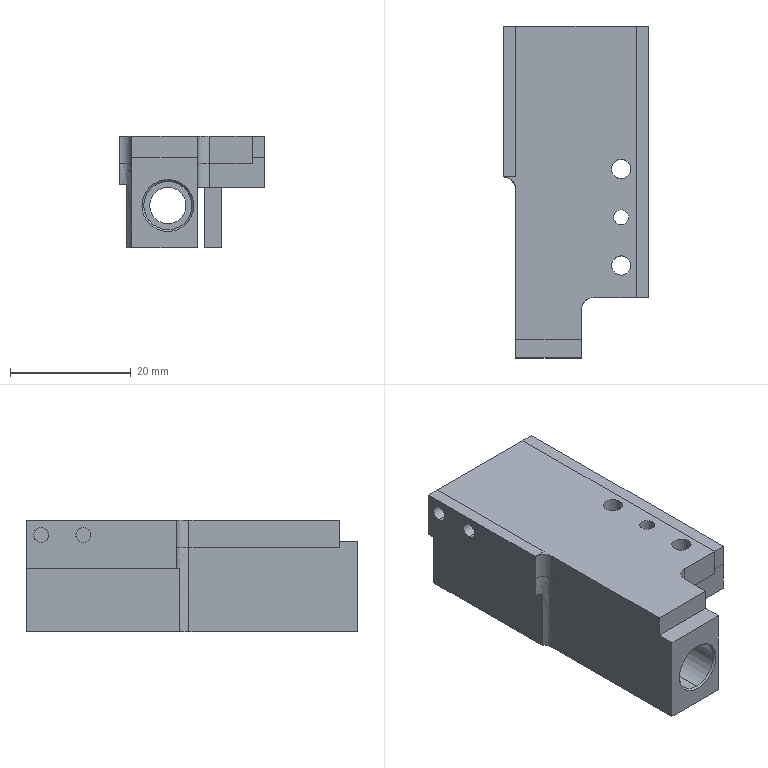NC program | NX | posted with a generic post | part box 24.15 x 55 x 18.5 mm
Lines 1 to 1747 of 2652:
N10 G17 G21 G94 G90
(FLOOR_WALL_COPY , TOOL : D63)
N12 T01 M6
N14 G54
N16 G17 G0 G90 X91.5 Y12.075 B0. C0. S6500 M3
N18 G43 Z30. H1
N20 Z8.571
N22 G94 G1 Z5.571 F1500.
N24 X86.5
N26 X-31.5
N28 X-36.5
N30 Z8.571
N32 G0 Z30.
N34 X91.5
N36 Z7.643
N38 G1 Z4.643
N40 X86.5
N42 X-31.5
N44 X-36.5
N46 Z7.643
N48 G0 Z30.
N50 X91.5
N52 Z6.714
N54 G1 Z3.714
N56 X86.5
N58 X-31.5
N60 X-36.5
N62 Z6.714
N64 G0 Z30.
N66 X91.5
N68 Z5.786
N70 G1 Z2.786
N72 X86.5
N74 X-31.5
N76 X-36.5
N78 Z5.786
N80 G0 Z30.
N82 X91.5
N84 Z4.857
N86 G1 Z1.857
N88 X86.5
N90 X-31.5
N92 X-36.5
N94 Z4.857
N96 G0 Z30.
N98 X91.5
N100 Z3.929
N102 G1 Z0.929
N104 X86.5
N106 X-31.5
N108 X-36.5
N110 Z3.929
N112 G0 Z30.
N114 X91.5
N116 Z3.
N118 G1 Z0.
N120 X86.5
N122 X-31.5
N124 X-36.5
N126 Z3.
N128 G0 Z30.
N130 M5
(FLOOR_WALL_1 , TOOL : D10)
N132 T10 M6
N134 G54
N136 G17 G0 G90 X34.979 Y-6. B0. C0. S9500 M3
N138 G43 Z30. H10
N140 Z-0.99
N142 G94 G1 X34.691 Y-5.5 F1000.
N144 G3 X33.825 Y-5. R1.
N146 G1 X-5. F3000.
N148 Y2.075
N150 X18.1
N152 Y6.075
N154 X50.
N156 Y-5.
N158 X33.825
N160 Y0.
N162 X22.649
N164 G3 X22.999 Y1.075 R5.
N166 G1 X45.
N168 Y0.
N170 X33.825
N172 G3 X32.959 Y-0.5 R1.
N174 G0 Z30.
N176 X34.979 Y-6.
N178 Z-1.98
N180 G1 X34.691 Y-5.5 F1000.
N182 G3 X33.825 Y-5. R1.
N184 G1 X-5. F3000.
N186 Y2.075
N188 X18.1
N190 Y6.075
N192 X50.
N194 Y-5.
N196 X33.825
N198 Y0.
N200 X22.649
N202 G3 X22.999 Y1.075 R5.
N204 G1 X45.
N206 Y0.
N208 X33.825
N210 G3 X32.959 Y-0.5 R1.
N212 G0 Z30.
N214 X34.979 Y-6.
N216 Z-2.97
N218 G1 X34.691 Y-5.5 F1000.
N220 G3 X33.825 Y-5. R1.
N222 G1 X-5. F3000.
N224 Y2.075
N226 X18.1
N228 Y6.075
N230 X50.
N232 Y-5.
N234 X33.825
N236 Y0.
N238 X22.649
N240 G3 X22.999 Y1.075 R5.
N242 G1 X45.
N244 Y0.
N246 X33.825
N248 G3 X32.959 Y-0.5 R1.
N250 G0 Z30.
N252 X34.979 Y-6.
N254 Z-3.96
N256 G1 X34.691 Y-5.5 F1000.
N258 G3 X33.825 Y-5. R1.
N260 G1 X-5. F3000.
N262 Y2.075
N264 X18.1
N266 Y6.075
N268 X50.
N270 Y-5.
N272 X33.825
N274 Y0.
N276 X22.649
N278 G3 X22.999 Y1.075 R5.
N280 G1 X45.
N282 Y0.
N284 X33.825
N286 G3 X32.959 Y-0.5 R1.
N288 G0 Z30.
N290 X34.979 Y-6.
N292 Z-4.95
N294 G1 X34.691 Y-5.5 F1000.
N296 G3 X33.825 Y-5. R1.
N298 G1 X-5. F3000.
N300 Y2.075
N302 X18.1
N304 Y6.075
N306 X50.
N308 Y-5.
N310 X33.825
N312 Y0.
N314 X22.649
N316 G3 X22.999 Y1.075 R5.
N318 G1 X45.
N320 Y0.
N322 X33.825
N324 G3 X32.959 Y-0.5 R1.
N326 G0 Z30.
N328 X34.979 Y-6.
N330 Z-5.94
N332 G1 X34.691 Y-5.5 F1000.
N334 G3 X33.825 Y-5. R1.
N336 G1 X-5. F3000.
N338 Y2.075
N340 X18.1
N342 Y6.075
N344 X50.
N346 Y-5.
N348 X33.825
N350 Y0.
N352 X22.649
N354 G3 X22.999 Y1.075 R5.
N356 G1 X45.
N358 Y0.
N360 X33.825
N362 G3 X32.959 Y-0.5 R1.
N364 G0 Z30.
N366 X34.979 Y-6.
N368 Z-6.93
N370 G1 X34.691 Y-5.5 F1000.
N372 G3 X33.825 Y-5. R1.
N374 G1 X-5. F3000.
N376 Y2.075
N378 X18.1
N380 Y6.075
N382 X50.
N384 Y-5.
N386 X33.825
N388 Y0.
N390 X22.649
N392 G3 X22.999 Y1.075 R5.
N394 G1 X45.
N396 Y0.
N398 X33.825
N400 G3 X32.959 Y-0.5 R1.
N402 G0 Z30.
N404 X34.979 Y-6.
N406 Z-7.92
N408 G1 X34.691 Y-5.5 F1000.
N410 G3 X33.825 Y-5. R1.
N412 G1 X-5. F3000.
N414 Y2.075
N416 X18.1
N418 Y6.075
N420 X50.
N422 Y-5.
N424 X33.825
N426 Y0.
N428 X22.649
N430 G3 X22.999 Y1.075 R5.
N432 G1 X45.
N434 Y0.
N436 X33.825
N438 G3 X32.959 Y-0.5 R1.
N440 G0 Z30.
N442 X34.979 Y-6.
N444 Z-8.91
N446 G1 X34.691 Y-5.5 F1000.
N448 G3 X33.825 Y-5. R1.
N450 G1 X-5. F3000.
N452 Y2.075
N454 X18.1
N456 Y6.075
N458 X50.
N460 Y-5.
N462 X33.825
N464 Y0.
N466 X22.649
N468 G3 X22.999 Y1.075 R5.
N470 G1 X45.
N472 Y0.
N474 X33.825
N476 G3 X32.959 Y-0.5 R1.
N478 G0 Z30.
N480 X34.979 Y-6.
N482 Z-9.9
N484 G1 X34.691 Y-5.5 F1000.
N486 G3 X33.825 Y-5. R1.
N488 G1 X-5. F3000.
N490 Y2.075
N492 X18.1
N494 Y6.075
N496 X50.
N498 Y-5.
N500 X33.825
N502 Y0.
N504 X22.649
N506 G3 X22.999 Y1.075 R5.
N508 G1 X45.
N510 Y0.
N512 X33.825
N514 G3 X32.959 Y-0.5 R1.
N516 G0 Z30.
(CAVITY_MILL , TOOL : D10)
N518 X-6.064 Y16.076
N520 Z0.5
N522 G1 Z-1. F1000.
N524 X-0.56 Y16.941
N526 G2 X-0.06 Y16.075 R1.
N528 G1 Y15.175 F3000.
N530 X13.
N532 X13.264 Y15.168
N534 G2 X13.773 Y15.116 R5.1
N536 G1 X15.811
N538 X15.812 Y14.989
N540 X15.84 Y14.816
N542 Y14.542
N544 Y14.38
N546 X15.826
N548 X15.784 Y14.399
N550 X15.777 Y14.352
N552 X15.9 Y14.27
N554 Y16.975
N556 X-0.06
N558 Y16.075
N560 G2 X-0.56 Y15.209 R1.
N562 G1 X-6.064 Y16.076
N564 Z0.5
N566 G0 X-6.065 Z-0.5
N568 G1 Z-2. F1000.
N570 X-0.56 Y16.941
N572 G2 X-0.06 Y16.075 R1.
N574 G1 Y15.175 F3000.
N576 X13.
N578 X13.264 Y15.168
N580 G2 X13.773 Y15.116 R5.1
N582 G1 X15.811
N584 X15.812 Y14.989
N586 X15.84 Y14.816
N588 Y14.542
N590 Y14.38
N592 X15.826
N594 X15.784 Y14.399
N596 X15.777 Y14.353
N598 X15.9 Y14.27
N600 Y16.975
N602 X-0.06
N604 Y16.075
N606 G2 X-0.56 Y15.209 R1.
N608 G1 X-6.065 Y16.076
N610 Z-0.5
N612 G0 X-6.067 Z-1.5
N614 G1 Z-3. F1000.
N616 X-0.56 Y16.941
N618 G2 X-0.06 Y16.075 R1.
N620 G1 Y15.175 F3000.
N622 X13.
N624 X13.264 Y15.168
N626 G2 X13.773 Y15.116 R5.1
N628 G1 X15.811
N630 X15.812 Y14.989
N632 X15.84 Y14.816
N634 Y14.542
N636 Y14.38
N638 X15.826
N640 X15.784 Y14.399
N642 X15.777 Y14.353
N644 X15.9 Y14.27
N646 Y16.975
N648 X-0.06
N650 Y16.075
N652 G2 X-0.56 Y15.209 R1.
N654 G1 X-6.067 Y16.076
N656 Z-1.5
N658 G0 X-6.069 Z-2.5
N660 G1 Z-4. F1000.
N662 X-0.56 Y16.941
N664 G2 X-0.06 Y16.075 R1.
N666 G1 Y15.175 F3000.
N668 X13.
N670 X13.264 Y15.168
N672 G2 X13.773 Y15.116 R5.1
N674 G1 X15.811
N676 X15.812 Y14.989
N678 X15.84 Y14.816
N680 Y14.542
N682 Y14.38
N684 X15.826
N686 X15.784 Y14.399
N688 X15.777 Y14.353
N690 X15.9 Y14.271
N692 Y16.975
N694 X-0.06
N696 Y16.075
N698 G2 X-0.56 Y15.209 R1.
N700 G1 X-6.069 Y16.076
N702 Z-2.5
N704 G0 X-6.07 Z-3.5
N706 G1 Z-5. F1000.
N708 X-0.56 Y16.941
N710 G2 X-0.06 Y16.075 R1.
N712 G1 Y15.175 F3000.
N714 X13.
N716 X13.216 Y15.173
N718 X13.264 Y15.168
N720 G2 X13.773 Y15.116 R5.1
N722 G1 X15.811
N724 X15.812 Y14.989
N726 X15.84 Y14.816
N728 Y14.542
N730 Y14.38
N732 X15.826
N734 X15.784 Y14.399
N736 X15.777 Y14.353
N738 X15.899 Y14.271
N740 X15.9 Y16.975
N742 X-0.06
N744 Y16.075
N746 G2 X-0.56 Y15.209 R1.
N748 G1 X-6.07 Y16.076
N750 Z-3.5
N752 G0 X-6.072 Z-4.5
N754 G1 Z-6. F1000.
N756 X-0.56 Y16.941
N758 G2 X-0.06 Y16.075 R1.
N760 G1 Y15.175 F3000.
N762 X13.
N764 X13.216 Y15.173
N766 X13.264 Y15.168
N768 G2 X13.773 Y15.116 R5.1
N770 G1 X15.811
N772 X15.812 Y14.989
N774 X15.84 Y14.816
N776 Y14.542
N778 Y14.38
N780 X15.826
N782 X15.784 Y14.399
N784 X15.777 Y14.353
N786 X15.899 Y14.272
N788 Y16.975
N790 X-0.06
N792 Y16.075
N794 G2 X-0.56 Y15.209 R1.
N796 G1 X-6.072 Y16.076
N798 Z-4.5
N800 G0 X-6.073 Z-5.5
N802 G1 Z-7. F1000.
N804 X-0.56 Y16.941
N806 G2 X-0.06 Y16.075 R1.
N808 G1 Y15.175 F3000.
N810 X13.
N812 X13.216 Y15.174
N814 X13.264 Y15.168
N816 G2 X13.773 Y15.116 R5.1
N818 G1 X15.811
N820 X15.812 Y14.989
N822 X15.84 Y14.816
N824 Y14.542
N826 Y14.38
N828 X15.826
N830 X15.784 Y14.399
N832 X15.777 Y14.353
N834 X15.899 Y14.273
N836 Y16.975
N838 X-0.06
N840 Y16.075
N842 G2 X-0.56 Y15.209 R1.
N844 G1 X-6.073 Y16.076
N846 Z-5.5
N848 G0 X-6.075 Z-6.5
N850 G1 Z-8. F1000.
N852 X-0.56 Y16.941
N854 G2 X-0.06 Y16.075 R1.
N856 G1 Y15.175 F3000.
N858 X13.
N860 X13.216 Y15.174
N862 X13.264 Y15.168
N864 G2 X13.773 Y15.116 R5.1
N866 G1 X15.811
N868 X15.812 Y14.989
N870 X15.84 Y14.816
N872 Y14.542
N874 Y14.38
N876 X15.826
N878 X15.784 Y14.399
N880 X15.777 Y14.353
N882 X15.898 Y14.273
N884 X15.899 Y16.975
N886 X-0.06
N888 Y16.075
N890 G2 X-0.56 Y15.209 R1.
N892 G1 X-6.075 Y16.076
N894 Z-6.5
N896 G0 X-6.076 Z-7.5
N898 G1 Z-9. F1000.
N900 X-0.56 Y16.941
N902 G2 X-0.06 Y16.075 R1.
N904 G1 Y15.175 F3000.
N906 X13.
N908 X13.216
N910 X13.264 Y15.168
N912 G2 X13.773 Y15.116 R5.1
N914 G1 X15.811
N916 X15.812 Y14.989
N918 X15.84 Y14.816
N920 Y14.542
N922 Y14.38
N924 X15.826
N926 X15.784 Y14.399
N928 X15.777 Y14.353
N930 X15.898 Y14.274
N932 X15.899 Y16.975
N934 X-0.06
N936 Y16.075
N938 G2 X-0.56 Y15.209 R1.
N940 G1 X-6.076 Y16.076
N942 Z-7.5
N944 G0 X-6.078 Z-8.5
N946 G1 Z-10. F1000.
N948 X-0.56 Y16.941
N950 G2 X-0.06 Y16.075 R1.
N952 G1 Y15.175 F3000.
N954 X13.288
N956 X15.9
N958 X15.899 Y16.975
N960 X-0.06
N962 Y16.075
N964 G2 X-0.56 Y15.209 R1.
N966 G1 X-6.078 Y16.076
N968 Z-8.5
N970 G0 X-6.079 Z-9.45
N972 G1 Z-10.95 F1000.
N974 X-0.56 Y16.941
N976 G2 X-0.06 Y16.075 R1.
N978 G1 Y15.175 F3000.
N980 X15.9
N982 X15.899 Y16.975
N984 X-0.06
N986 Y16.075
N988 G2 X-0.56 Y15.209 R1.
N990 G1 X-6.079 Y16.076
N992 Z-9.45
N994 G0 X-6.081 Z-10.4
N996 G1 Z-11.9 F1000.
N998 X-0.56 Y16.941
N1000 G2 X-0.06 Y16.075 R1.
N1002 G1 Y15.175 F3000.
N1004 X15.9
N1006 X15.899 Y16.975
N1008 X-0.06
N1010 Y16.075
N1012 G2 X-0.56 Y15.209 R1.
N1014 G1 X-6.081 Y16.076
N1016 Z-10.4
N1018 G0 Z30.
N1020 M5
(CAVITY_MILL_COPY , TOOL : D6)
N1022 T06 M6
N1024 G54
N1026 G17 G0 G90 X16.8 Y15.798 B0. C0. S9500 M3
N1028 G43 Z30. H6
N1030 Z0.5
N1032 G94 G1 Z-0.5 F1000.
N1034 X17.5 Y16.202
N1036 G3 X18. Y17.069 R1.
N1038 G1 Y19.075 F2000.
N1040 X15.994
N1042 G3 X15.127 Y18.575 R1.
N1044 G1 X14.723 Y17.875
N1046 Z0.5
N1048 G0 Z30.
N1050 X16.8 Y15.798
N1052 Z0.
N1054 G1 Z-1. F1000.
N1056 X17.5 Y16.202
N1058 G3 X18. Y17.068 R1.
N1060 G1 Y19.075 F2000.
N1062 X15.993
N1064 G3 X15.127 Y18.575 R1.
N1066 G1 X14.723 Y17.875
N1068 Z0.
N1070 G0 X16.8 Y15.798 Z-0.5
N1072 G1 Z-1.5 F1000.
N1074 X17.5 Y16.202
N1076 G3 X18. Y17.068 R1.
N1078 G1 Y19.075 F2000.
N1080 X15.993
N1082 G3 X15.127 Y18.575 R1.
N1084 G1 X14.723 Y17.875
N1086 Z-0.5
N1088 G0 X16.8 Y15.798 Z-1.
N1090 G1 Z-2. F1000.
N1092 X17.5 Y16.202
N1094 G3 X18. Y17.068 R1.
N1096 G1 Y19.075 F2000.
N1098 X15.993
N1100 G3 X15.127 Y18.575 R1.
N1102 G1 X14.723 Y17.875
N1104 Z-1.
N1106 G0 X16.8 Y15.798 Z-1.5
N1108 G1 Z-2.5 F1000.
N1110 X17.5 Y16.202
N1112 G3 X18. Y17.068 R1.
N1114 G1 Y19.075 F2000.
N1116 X15.993
N1118 G3 X15.127 Y18.575 R1.
N1120 G1 X14.723 Y17.875
N1122 Z-1.5
N1124 G0 X16.8 Y15.798 Z-2.
N1126 G1 Z-3. F1000.
N1128 X17.5 Y16.202
N1130 G3 X18. Y17.068 R1.
N1132 G1 Y19.075 F2000.
N1134 X15.993
N1136 G3 X15.127 Y18.575 R1.
N1138 G1 X14.723 Y17.875
N1140 Z-2.
N1142 G0 X16.8 Y15.798 Z-2.5
N1144 G1 Z-3.5 F1000.
N1146 X17.5 Y16.202
N1148 G3 X18. Y17.068 R1.
N1150 G1 Y19.075 F2000.
N1152 X15.993
N1154 G3 X15.127 Y18.575 R1.
N1156 G1 X14.723 Y17.875
N1158 Z-2.5
N1160 G0 X16.8 Y15.798 Z-3.
N1162 G1 Z-4. F1000.
N1164 X17.5 Y16.202
N1166 G3 X18. Y17.068 R1.
N1168 G1 Y19.075 F2000.
N1170 X15.993
N1172 G3 X15.127 Y18.575 R1.
N1174 G1 X14.723 Y17.875
N1176 Z-3.
N1178 G0 X16.8 Y15.798 Z-3.5
N1180 G1 Z-4.5 F1000.
N1182 X17.5 Y16.202
N1184 G3 X18. Y17.068 R1.
N1186 G1 Y19.075 F2000.
N1188 X15.993
N1190 G3 X15.127 Y18.575 R1.
N1192 G1 X14.723 Y17.875
N1194 Z-3.5
N1196 G0 X16.8 Y15.798 Z-4.
N1198 G1 Z-5. F1000.
N1200 X17.5 Y16.202
N1202 G3 X18. Y17.068 R1.
N1204 G1 Y19.075 F2000.
N1206 X15.993
N1208 G3 X15.127 Y18.575 R1.
N1210 G1 X14.723 Y17.875
N1212 Z-4.
N1214 G0 X16.8 Y15.798 Z-4.5
N1216 G1 Z-5.5 F1000.
N1218 X17.5 Y16.202
N1220 G3 X18. Y17.068 R1.
N1222 G1 Y19.075 F2000.
N1224 X15.993
N1226 G3 X15.127 Y18.575 R1.
N1228 G1 X14.723 Y17.875
N1230 Z-4.5
N1232 G0 X16.8 Y15.798 Z-5.
N1234 G1 Z-6. F1000.
N1236 X17.5 Y16.202
N1238 G3 X18. Y17.068 R1.
N1240 G1 Y19.075 F2000.
N1242 X15.993
N1244 G3 X15.127 Y18.575 R1.
N1246 G1 X14.723 Y17.875
N1248 Z-5.
N1250 G0 X16.8 Y15.798 Z-5.5
N1252 G1 Z-6.5 F1000.
N1254 X17.5 Y16.202
N1256 G3 X18. Y17.068 R1.
N1258 G1 Y19.075 F2000.
N1260 X15.993
N1262 G3 X15.127 Y18.575 R1.
N1264 G1 X14.723 Y17.875
N1266 Z-5.5
N1268 G0 X16.8 Y15.798 Z-6.
N1270 G1 Z-7. F1000.
N1272 X17.5 Y16.202
N1274 G3 X18. Y17.068 R1.
N1276 G1 Y19.075 F2000.
N1278 X15.993
N1280 G3 X15.127 Y18.575 R1.
N1282 G1 X14.723 Y17.875
N1284 Z-6.
N1286 G0 X16.8 Y15.798 Z-6.5
N1288 G1 Z-7.5 F1000.
N1290 X17.5 Y16.202
N1292 G3 X18. Y17.068 R1.
N1294 G1 Y19.075 F2000.
N1296 X15.993
N1298 G3 X15.127 Y18.575 R1.
N1300 G1 X14.723 Y17.875
N1302 Z-6.5
N1304 G0 X16.8 Y15.798 Z-7.
N1306 G1 Z-8. F1000.
N1308 X17.5 Y16.202
N1310 G3 X18. Y17.068 R1.
N1312 G1 Y19.075 F2000.
N1314 X15.993
N1316 G3 X15.127 Y18.575 R1.
N1318 G1 X14.723 Y17.875
N1320 Z-7.
N1322 G0 X16.8 Y15.798 Z-7.5
N1324 G1 Z-8.5 F1000.
N1326 X17.5 Y16.202
N1328 G3 X18. Y17.068 R1.
N1330 G1 Y19.075 F2000.
N1332 X15.993
N1334 G3 X15.127 Y18.575 R1.
N1336 G1 X14.723 Y17.875
N1338 Z-7.5
N1340 G0 X16.8 Y15.798 Z-8.
N1342 G1 Z-9. F1000.
N1344 X17.5 Y16.202
N1346 G3 X18. Y17.068 R1.
N1348 G1 Y19.075 F2000.
N1350 X15.993
N1352 G3 X15.127 Y18.575 R1.
N1354 G1 X14.723 Y17.875
N1356 Z-8.
N1358 G0 X16.8 Y15.798 Z-8.5
N1360 G1 Z-9.5 F1000.
N1362 X17.5 Y16.202
N1364 G3 X18. Y17.068 R1.
N1366 G1 Y19.075 F2000.
N1368 X15.993
N1370 G3 X15.127 Y18.575 R1.
N1372 G1 X14.723 Y17.875
N1374 Z-8.5
N1376 G0 X16.8 Y15.798 Z-9.
N1378 G1 Z-10. F1000.
N1380 X17.5 Y16.202
N1382 G3 X18. Y17.068 R1.
N1384 G1 Y19.075 F2000.
N1386 X15.993
N1388 G3 X15.127 Y18.575 R1.
N1390 G1 X14.723 Y17.875
N1392 Z-9.
N1394 G0 X16.8 Y15.797 Z-9.5
N1396 G1 Z-10.5 F1000.
N1398 X17.5 Y16.202
N1400 G3 X18. Y17.068 R1.
N1402 G1 Y19.075 F2000.
N1404 X15.993
N1406 G3 X15.127 Y18.575 R1.
N1408 G1 X14.722 Y17.875
N1410 Z-9.5
N1412 G0 X16.8 Y15.797 Z-10.
N1414 G1 Z-11. F1000.
N1416 X17.5 Y16.202
N1418 G3 X18. Y17.068 R1.
N1420 G1 Y19.075 F2000.
N1422 X15.993
N1424 G3 X15.127 Y18.575 R1.
N1426 G1 X14.722 Y17.875
N1428 Z-10.
N1430 G0 X16.8 Y15.797 Z-10.5
N1432 G1 Z-11.5 F1000.
N1434 X17.5 Y16.202
N1436 G3 X18. Y17.068 R1.
N1438 G1 Y19.075 F2000.
N1440 X15.993
N1442 G3 X15.127 Y18.575 R1.
N1444 G1 X14.722 Y17.875
N1446 Z-10.5
N1448 G0 X16.8 Y15.797 Z-11.
N1450 G1 Z-12. F1000.
N1452 X17.5 Y16.201
N1454 G3 X18. Y17.067 R1.
N1456 G1 Y19.075 F2000.
N1458 X15.992
N1460 G3 X15.126 Y18.575 R1.
N1462 G1 X14.722 Y17.875
N1464 Z-11.
N1466 G0 Z30.
N1468 X16.8 Y15.979
N1470 Z0.5
N1472 G1 Z-0.5 F1000.
N1474 X17.409 Y12.975
N1476 G2 X17.923 Y12.118 R1.
N1478 G1 X17.939 Y11.219 F2000.
N1480 X17.936 Y11.155
N1482 X18. Y11.16
N1484 Y14.082
N1486 G3 X17.515 Y13.702 R0.5
N1488 G2 X17.327 Y13.25 R1.563
N1490 G3 X17.269 Y13.016 R0.5
N1492 G1 X17.911
N1494 X17.923 Y12.118
N1496 G2 X17.438 Y11.243 R1.
N1498 G1 Z0.5
N1500 G0 Z30.
N1502 X16.8 Y15.979
N1504 Z0.
N1506 G1 Z-1. F1000.
N1508 X17.409 Y12.975
N1510 G2 X17.923 Y12.118 R1.
N1512 G1 X17.939 Y11.219 F2000.
N1514 X17.936 Y11.155
N1516 X18. Y11.16
N1518 Y14.082
N1520 G3 X17.515 Y13.702 R0.5
N1522 G2 X17.327 Y13.25 R1.563
N1524 G3 X17.269 Y13.016 R0.5
N1526 G1 X17.911
N1528 X17.923 Y12.118
N1530 G2 X17.438 Y11.243 R1.
N1532 G1 Z0.
N1534 G0 X16.8 Y15.979 Z-0.5
N1536 G1 Z-1.5 F1000.
N1538 X17.409 Y12.975
N1540 G2 X17.923 Y12.118 R1.
N1542 G1 X17.939 Y11.219 F2000.
N1544 X17.936 Y11.155
N1546 X18. Y11.16
N1548 Y14.082
N1550 G3 X17.515 Y13.702 R0.5
N1552 G2 X17.327 Y13.25 R1.563
N1554 G3 X17.269 Y13.016 R0.5
N1556 G1 X17.911
N1558 X17.923 Y12.118
N1560 G2 X17.438 Y11.243 R1.
N1562 G1 Z-0.5
N1564 G0 X16.8 Y15.979 Z-1.
N1566 G1 Z-2. F1000.
N1568 X17.409 Y12.975
N1570 G2 X17.923 Y12.118 R1.
N1572 G1 X17.939 Y11.219 F2000.
N1574 X17.936 Y11.155
N1576 X18. Y11.16
N1578 Y14.082
N1580 G3 X17.515 Y13.702 R0.5
N1582 G2 X17.327 Y13.25 R1.563
N1584 G3 X17.269 Y13.016 R0.5
N1586 G1 X17.911
N1588 X17.923 Y12.118
N1590 G2 X17.438 Y11.243 R1.
N1592 G1 Z-1.
N1594 G0 X16.8 Y15.979 Z-1.5
N1596 G1 Z-2.5 F1000.
N1598 X17.409 Y12.975
N1600 G2 X17.923 Y12.118 R1.
N1602 G1 X17.939 Y11.219 F2000.
N1604 X17.936 Y11.155
N1606 X18. Y11.16
N1608 Y14.082
N1610 G3 X17.515 Y13.702 R0.5
N1612 G2 X17.327 Y13.25 R1.563
N1614 G3 X17.269 Y13.016 R0.5
N1616 G1 X17.911
N1618 X17.923 Y12.118
N1620 G2 X17.438 Y11.243 R1.
N1622 G1 Z-1.5
N1624 G0 X16.8 Y15.979 Z-2.
N1626 G1 Z-3. F1000.
N1628 X17.409 Y12.975
N1630 G2 X17.923 Y12.118 R1.
N1632 G1 X17.939 Y11.219 F2000.
N1634 X17.936 Y11.155
N1636 X18. Y11.16
N1638 Y14.082
N1640 G3 X17.515 Y13.702 R0.5
N1642 G2 X17.327 Y13.25 R1.563
N1644 G3 X17.269 Y13.016 R0.5
N1646 G1 X17.911
N1648 X17.923 Y12.118
N1650 G2 X17.438 Y11.243 R1.
N1652 G1 Z-2.
N1654 G0 X16.8 Y15.979 Z-2.5
N1656 G1 Z-3.5 F1000.
N1658 X17.409 Y12.975
N1660 G2 X17.923 Y12.118 R1.
N1662 G1 X17.939 Y11.219 F2000.
N1664 X17.936 Y11.155
N1666 X18. Y11.16
N1668 Y14.088
N1670 G3 X17.514 Y13.707 R0.5
N1672 G2 X17.325 Y13.249 R1.563
N1674 G3 X17.267 Y13.016 R0.5
N1676 G1 X17.911
N1678 X17.923 Y12.118
N1680 G2 X17.438 Y11.243 R1.
N1682 G1 Z-2.5
N1684 G0 X16.8 Y15.979 Z-3.
N1686 G1 Z-4. F1000.
N1688 X17.409 Y12.975
N1690 G2 X17.923 Y12.118 R1.
N1692 G1 X17.939 Y11.219 F2000.
N1694 X17.936 Y11.155
N1696 X18. Y11.16
N1698 Y14.088
N1700 G3 X17.514 Y13.707 R0.5
N1702 G2 X17.325 Y13.249 R1.563
N1704 G3 X17.267 Y13.016 R0.5
N1706 G1 X17.911
N1708 X17.923 Y12.118
N1710 G2 X17.438 Y11.243 R1.
N1712 G1 Z-3.
N1714 G0 X16.8 Y15.979 Z-3.5
N1716 G1 Z-4.5 F1000.
N1718 X17.409 Y12.975
N1720 G2 X17.923 Y12.118 R1.
N1722 G1 X17.939 Y11.219 F2000.
N1724 X17.936 Y11.155
N1726 X18. Y11.16
N1728 Y14.088
N1730 G3 X17.514 Y13.707 R0.5
N1732 G2 X17.325 Y13.249 R1.563
N1734 G3 X17.267 Y13.016 R0.5
N1736 G1 X17.911
N1738 X17.923 Y12.118
N1740 G2 X17.438 Y11.243 R1.
N1742 G1 Z-3.5
N1744 G0 X16.8 Y15.979 Z-4.
N1746 G1 Z-5. F1000.
N1748 X17.409 Y12.975
N1750 G2 X17.923 Y12.118 R1.
N1752 G1 X17.939 Y11.219 F2000.
N1754 X17.936 Y11.155
N1756 X18. Y11.16
N1758 Y14.088
N1760 G3 X17.514 Y13.707 R0.5
N1762 G2 X17.325 Y13.249 R1.563
N1764 G3 X17.267 Y13.016 R0.5
N1766 G1 X17.911
N1768 X17.923 Y12.118
N1770 G2 X17.438 Y11.243 R1.
N1772 G1 Z-4.
N1774 G0 X16.8 Y15.979 Z-4.5
N1776 G1 Z-5.5 F1000.
N1778 X17.409 Y12.975
N1780 G2 X17.923 Y12.118 R1.
N1782 G1 X17.939 Y11.219 F2000.
N1784 X17.936 Y11.155
N1786 X18. Y11.16
N1788 Y14.088
N1790 G3 X17.514 Y13.707 R0.5
N1792 G2 X17.325 Y13.249 R1.563
N1794 G3 X17.267 Y13.016 R0.5
N1796 G1 X17.911
N1798 X17.923 Y12.118
N1800 G2 X17.438 Y11.243 R1.
N1802 G1 Z-4.5
N1804 G0 X16.8 Y15.979 Z-5.
N1806 G1 Z-6. F1000.
N1808 X17.409 Y12.975
N1810 G2 X17.923 Y12.118 R1.
N1812 G1 X17.939 Y11.219 F2000.
N1814 X17.936 Y11.155
N1816 X18. Y11.16
N1818 Y14.088
N1820 G3 X17.514 Y13.707 R0.5
N1822 G2 X17.325 Y13.249 R1.563
N1824 G3 X17.267 Y13.016 R0.5
N1826 G1 X17.911
N1828 X17.923 Y12.118
N1830 G2 X17.438 Y11.243 R1.
N1832 G1 Z-5.
N1834 G0 X16.8 Y15.979 Z-5.5
N1836 G1 Z-6.5 F1000.
N1838 X17.409 Y12.975
N1840 G2 X17.923 Y12.118 R1.
N1842 G1 X17.939 Y11.219 F2000.
N1844 X17.936 Y11.155
N1846 X18. Y11.16
N1848 Y14.087
N1850 G3 X17.514 Y13.706 R0.5
N1852 G2 X17.325 Y13.249 R1.563
N1854 G3 X17.267 Y13.016 R0.5
N1856 G1 X17.911
N1858 X17.923 Y12.118
N1860 G2 X17.438 Y11.243 R1.
N1862 G1 Z-5.5
N1864 G0 X16.8 Y15.979 Z-6.
N1866 G1 Z-7. F1000.
N1868 X17.409 Y12.975
N1870 G2 X17.923 Y12.118 R1.
N1872 G1 X17.939 Y11.219 F2000.
N1874 X17.936 Y11.155
N1876 X18. Y11.16
N1878 Y14.088
N1880 G3 X17.514 Y13.707 R0.5
N1882 G2 X17.325 Y13.249 R1.563
N1884 G3 X17.267 Y13.016 R0.5
N1886 G1 X17.911
N1888 X17.923 Y12.118
N1890 G2 X17.438 Y11.243 R1.
N1892 G1 Z-6.
N1894 G0 X16.8 Y15.979 Z-6.5
N1896 G1 Z-7.5 F1000.
N1898 X17.409 Y12.975
N1900 G2 X17.923 Y12.118 R1.
N1902 G1 X17.939 Y11.219 F2000.
N1904 X17.936 Y11.155
N1906 X18. Y11.16
N1908 Y14.088
N1910 G3 X17.514 Y13.707 R0.5
N1912 G2 X17.325 Y13.249 R1.563
N1914 G3 X17.267 Y13.016 R0.5
N1916 G1 X17.911
N1918 X17.923 Y12.118
N1920 G2 X17.438 Y11.243 R1.
N1922 G1 Z-6.5
N1924 G0 X16.8 Y15.979 Z-7.
N1926 G1 Z-8. F1000.
N1928 X17.409 Y12.975
N1930 G2 X17.923 Y12.118 R1.
N1932 G1 X17.939 Y11.219 F2000.
N1934 X17.936 Y11.155
N1936 X18. Y11.16
N1938 Y14.088
N1940 G3 X17.514 Y13.707 R0.5
N1942 G2 X17.325 Y13.249 R1.563
N1944 G3 X17.267 Y13.016 R0.5
N1946 G1 X17.911
N1948 X17.923 Y12.118
N1950 G2 X17.438 Y11.243 R1.
N1952 G1 Z-7.
N1954 G0 X16.8 Y15.979 Z-7.5
N1956 G1 Z-8.5 F1000.
N1958 X17.409 Y12.975
N1960 G2 X17.923 Y12.118 R1.
N1962 G1 X17.939 Y11.219 F2000.
N1964 X17.936 Y11.155
N1966 X18. Y11.16
N1968 Y14.088
N1970 G3 X17.514 Y13.707 R0.5
N1972 G2 X17.325 Y13.249 R1.563
N1974 G3 X17.267 Y13.016 R0.5
N1976 G1 X17.911
N1978 X17.923 Y12.118
N1980 G2 X17.438 Y11.243 R1.
N1982 G1 Z-7.5
N1984 G0 X16.8 Y15.979 Z-8.
N1986 G1 Z-9. F1000.
N1988 X17.409 Y12.975
N1990 G2 X17.923 Y12.118 R1.
N1992 G1 X17.939 Y11.219 F2000.
N1994 X17.936 Y11.155
N1996 X18. Y11.16
N1998 Y14.088
N2000 G3 X17.514 Y13.707 R0.5
N2002 G2 X17.325 Y13.249 R1.563
N2004 G3 X17.267 Y13.016 R0.5
N2006 G1 X17.911
N2008 X17.923 Y12.118
N2010 G2 X17.438 Y11.243 R1.
N2012 G1 Z-8.
N2014 G0 X16.8 Y15.979 Z-8.5
N2016 G1 Z-9.5 F1000.
N2018 X17.409 Y12.975
N2020 G2 X17.923 Y12.118 R1.
N2022 G1 X17.939 Y11.219 F2000.
N2024 X17.936 Y11.155
N2026 X18. Y11.16
N2028 Y14.088
N2030 G3 X17.514 Y13.707 R0.5
N2032 G2 X17.325 Y13.249 R1.563
N2034 G3 X17.267 Y13.016 R0.5
N2036 G1 X17.911
N2038 X17.923 Y12.118
N2040 G2 X17.438 Y11.243 R1.
N2042 G1 Z-8.5
N2044 G0 X16.8 Y15.979 Z-9.
N2046 G1 Z-10. F1000.
N2048 X17.409 Y12.975
N2050 G2 X17.923 Y12.118 R1.
N2052 G1 X17.939 Y11.219 F2000.
N2054 X17.936 Y11.155
N2056 X18. Y11.16
N2058 Y14.088
N2060 G3 X17.514 Y13.707 R0.5
N2062 G2 X17.325 Y13.249 R1.563
N2064 G3 X17.267 Y13.016 R0.5
N2066 G1 X17.911
N2068 X17.923 Y12.118
N2070 G2 X17.438 Y11.243 R1.
N2072 G1 Z-9.
N2074 G0 X14.723 Y14.275 Z-9.5
N2076 G1 Z-10.5 F1000.
N2078 X15.128 Y13.575
N2080 G3 X15.994 Y13.075 R1.
N2082 G1 X18. F2000.
N2084 Y15.081
N2086 G3 X17.5 Y15.947 R1.
N2088 G1 X16.8 Y16.352
N2090 Z-9.5
N2092 G0 X14.723 Y14.275 Z-10.
N2094 G1 Z-11. F1000.
N2096 X15.128 Y13.575
N2098 G3 X15.994 Y13.075 R1.
N2100 G1 X18. F2000.
N2102 Y15.081
N2104 G3 X17.5 Y15.947 R1.
N2106 G1 X16.8 Y16.352
N2108 Z-10.
N2110 G0 X14.723 Y14.275 Z-10.5
N2112 G1 Z-11.5 F1000.
N2114 X15.128 Y13.575
N2116 G3 X15.994 Y13.075 R1.
N2118 G1 X18. F2000.
N2120 Y15.081
N2122 G3 X17.5 Y15.947 R1.
N2124 G1 X16.8 Y16.352
N2126 Z-10.5
N2128 G0 X14.723 Y14.275 Z-11.
N2130 G1 Z-12. F1000.
N2132 X15.128 Y13.575
N2134 G3 X15.994 Y13.075 R1.
N2136 G1 X18. F2000.
N2138 Y15.081
N2140 G3 X17.5 Y15.947 R1.
N2142 G1 X16.8 Y16.352
N2144 Z-11.
N2146 G0 Z30.
N2148 X18.622 Y7.153
N2150 Z0.5
N2152 G1 Z-0.5 F1000.
N2154 X18.003 Y10.197
N2156 G2 X17.753 Y10.131 R0.5
N2158 G1 X17.314 Y10.132 F2000.
N2160 G3 X17.38 Y9.883 R0.5
N2162 X18.657 Y8.592 R3.5
N2164 X19.295 Y8.707 R0.5
N2166 G2 X18.191 Y10.121 R3.
N2168 G1 X18.142 Y10.13
N2170 X17.753 Y10.131
N2172 G2 X17.321 Y10.382 R0.5
N2174 G1 X18.622 Y7.153
N2176 Z0.5
N2178 G0 Z30.
N2180 Z0.
N2182 G1 Z-1. F1000.
N2184 X18.003 Y10.197
N2186 G2 X17.753 Y10.131 R0.5
N2188 G1 X17.314 Y10.132 F2000.
N2190 G3 X17.38 Y9.883 R0.5
N2192 X18.657 Y8.592 R3.5
N2194 X19.295 Y8.707 R0.5
N2196 G2 X18.191 Y10.121 R3.
N2198 G1 X18.142 Y10.13
N2200 X17.753 Y10.131
N2202 G2 X17.321 Y10.382 R0.5
N2204 G1 X18.622 Y7.153
N2206 Z0.
N2208 G0 Z-0.5
N2210 G1 Z-1.5 F1000.
N2212 X18.003 Y10.197
N2214 G2 X17.753 Y10.131 R0.5
N2216 G1 X17.314 Y10.132 F2000.
N2218 G3 X17.38 Y9.883 R0.5
N2220 X18.657 Y8.592 R3.5
N2222 X19.295 Y8.707 R0.5
N2224 G2 X18.191 Y10.121 R3.
N2226 G1 X18.142 Y10.13
N2228 X17.753 Y10.131
N2230 G2 X17.321 Y10.382 R0.5
N2232 G1 X18.622 Y7.153
N2234 Z-0.5
N2236 G0 Z-1.
N2238 G1 Z-2. F1000.
N2240 X18.003 Y10.197
N2242 G2 X17.753 Y10.131 R0.5
N2244 G1 X17.314 Y10.132 F2000.
N2246 G3 X17.38 Y9.883 R0.5
N2248 X18.657 Y8.592 R3.5
N2250 X19.295 Y8.707 R0.5
N2252 G2 X18.191 Y10.121 R3.
N2254 G1 X18.142 Y10.13
N2256 X17.753 Y10.131
N2258 G2 X17.321 Y10.382 R0.5
N2260 G1 X18.622 Y7.153
N2262 Z-1.
N2264 G0 Z-1.5
N2266 G1 Z-2.5 F1000.
N2268 X18.003 Y10.197
N2270 G2 X17.753 Y10.131 R0.5
N2272 G1 X17.314 Y10.132 F2000.
N2274 G3 X17.38 Y9.883 R0.5
N2276 X18.657 Y8.592 R3.5
N2278 X19.295 Y8.707 R0.5
N2280 G2 X18.191 Y10.121 R3.
N2282 G1 X18.142 Y10.13
N2284 X17.753 Y10.131
N2286 G2 X17.321 Y10.382 R0.5
N2288 G1 X18.622 Y7.153
N2290 Z-1.5
N2292 G0 Z-2.
N2294 G1 Z-3. F1000.
N2296 X18.003 Y10.197
N2298 G2 X17.753 Y10.131 R0.5
N2300 G1 X17.314 Y10.132 F2000.
N2302 G3 X17.38 Y9.883 R0.5
N2304 X18.657 Y8.592 R3.5
N2306 X19.295 Y8.707 R0.5
N2308 G2 X18.191 Y10.121 R3.
N2310 G1 X18.142 Y10.13
N2312 X17.753 Y10.131
N2314 G2 X17.321 Y10.382 R0.5
N2316 G1 X18.622 Y7.153
N2318 Z-2.
N2320 G0 X18.621 Y7.152 Z-2.5
N2322 G1 Z-3.5 F1000.
N2324 X18.003 Y10.197
N2326 G2 X17.753 Y10.131 R0.5
N2328 G1 X17.313 Y10.132 F2000.
N2330 G3 X17.379 Y9.883 R0.5
N2332 X18.657 Y8.592 R3.5
N2334 X19.295 Y8.707 R0.5
N2336 G2 X18.191 Y10.121 R3.
N2338 G1 X18.142 Y10.13
N2340 X17.753 Y10.131
N2342 G2 X17.321 Y10.382 R0.5
N2344 G1 X18.621 Y7.152
N2346 Z-2.5
N2348 G0 Z-3.
N2350 G1 Z-4. F1000.
N2352 X18.003 Y10.197
N2354 G2 X17.753 Y10.131 R0.5
N2356 G1 X17.313 Y10.132 F2000.
N2358 G3 X17.379 Y9.883 R0.5
N2360 X18.657 Y8.592 R3.5
N2362 X19.295 Y8.707 R0.5
N2364 G2 X18.191 Y10.121 R3.
N2366 G1 X18.142 Y10.13
N2368 X17.753 Y10.131
N2370 G2 X17.321 Y10.382 R0.5
N2372 G1 X18.621 Y7.152
N2374 Z-3.
N2376 G0 Z-3.5
N2378 G1 Z-4.5 F1000.
N2380 X18.003 Y10.197
N2382 G2 X17.753 Y10.131 R0.5
N2384 G1 X17.313 Y10.132 F2000.
N2386 G3 X17.379 Y9.883 R0.5
N2388 X18.657 Y8.592 R3.5
N2390 X19.295 Y8.707 R0.5
N2392 G2 X18.191 Y10.121 R3.
N2394 G1 X18.142 Y10.13
N2396 X17.753 Y10.131
N2398 G2 X17.321 Y10.382 R0.5
N2400 G1 X18.621 Y7.152
N2402 Z-3.5
N2404 G0 Z-4.
N2406 G1 Z-5. F1000.
N2408 X18.003 Y10.197
N2410 G2 X17.753 Y10.131 R0.5
N2412 G1 X17.313 Y10.132 F2000.
N2414 G3 X17.379 Y9.883 R0.5
N2416 X18.657 Y8.592 R3.5
N2418 X19.295 Y8.707 R0.5
N2420 G2 X18.191 Y10.121 R3.
N2422 G1 X18.142 Y10.13
N2424 X17.753 Y10.131
N2426 G2 X17.321 Y10.382 R0.5
N2428 G1 X18.621 Y7.152
N2430 Z-4.
N2432 G0 Z-4.5
N2434 G1 Z-5.5 F1000.
N2436 X18.003 Y10.197
N2438 G2 X17.753 Y10.131 R0.5
N2440 G1 X17.313 Y10.132 F2000.
N2442 G3 X17.379 Y9.883 R0.5
N2444 X18.657 Y8.592 R3.5
N2446 X19.295 Y8.707 R0.5
N2448 G2 X18.191 Y10.121 R3.
N2450 G1 X18.142 Y10.13
N2452 X17.753 Y10.131
N2454 G2 X17.321 Y10.382 R0.5
N2456 G1 X18.621 Y7.152
N2458 Z-4.5
N2460 G0 Z-5.
N2462 G1 Z-6. F1000.
N2464 X18.003 Y10.197
N2466 G2 X17.753 Y10.131 R0.5
N2468 G1 X17.313 Y10.132 F2000.
N2470 G3 X17.379 Y9.883 R0.5
N2472 X18.657 Y8.592 R3.5
N2474 X19.295 Y8.707 R0.5
N2476 G2 X18.191 Y10.121 R3.
N2478 G1 X18.142 Y10.13
N2480 X17.753 Y10.131
N2482 G2 X17.321 Y10.382 R0.5
N2484 G1 X18.621 Y7.152
N2486 Z-5.
N2488 G0 Z-5.5
N2490 G1 Z-6.5 F1000.
N2492 X18.003 Y10.197
N2494 G2 X17.753 Y10.131 R0.5
N2496 G1 X17.313 Y10.132 F2000.
N2498 G3 X17.379 Y9.883 R0.5
N2500 X18.657 Y8.592 R3.5
N2502 X19.295 Y8.707 R0.5
N2504 G2 X18.191 Y10.121 R3.
N2506 G1 X18.142 Y10.13
N2508 X17.753 Y10.131
N2510 G2 X17.321 Y10.382 R0.5
N2512 G1 X18.621 Y7.152
N2514 Z-5.5
N2516 G0 Z-6.
N2518 G1 Z-7. F1000.
N2520 X18.003 Y10.197
N2522 G2 X17.753 Y10.131 R0.5
N2524 G1 X17.313 Y10.132 F2000.
N2526 G3 X17.379 Y9.883 R0.5
N2528 X18.657 Y8.592 R3.5
N2530 X19.295 Y8.707 R0.5
N2532 G2 X18.191 Y10.121 R3.
N2534 G1 X18.142 Y10.13
N2536 X17.753 Y10.131
N2538 G2 X17.321 Y10.382 R0.5
N2540 G1 X18.621 Y7.152
N2542 Z-6.
N2544 G0 Z-6.5
N2546 G1 Z-7.5 F1000.
N2548 X18.003 Y10.197
N2550 G2 X17.753 Y10.131 R0.5
N2552 G1 X17.313 Y10.132 F2000.
N2554 G3 X17.379 Y9.883 R0.5
N2556 X18.657 Y8.592 R3.5
N2558 X19.295 Y8.707 R0.5
N2560 G2 X18.191 Y10.121 R3.
N2562 G1 X18.142 Y10.13
N2564 X17.753 Y10.131
N2566 G2 X17.321 Y10.382 R0.5
N2568 G1 X18.621 Y7.152
N2570 Z-6.5
N2572 G0 Z-7.
N2574 G1 Z-8. F1000.
N2576 X18.003 Y10.197
N2578 G2 X17.753 Y10.131 R0.5
N2580 G1 X17.313 Y10.132 F2000.
N2582 G3 X17.379 Y9.883 R0.5
N2584 X18.657 Y8.592 R3.5
N2586 X19.295 Y8.707 R0.5
N2588 G2 X18.191 Y10.121 R3.
N2590 G1 X18.142 Y10.13
N2592 X17.753 Y10.131
N2594 G2 X17.321 Y10.382 R0.5
N2596 G1 X18.621 Y7.152
N2598 Z-7.
N2600 G0 Z-7.5
N2602 G1 Z-8.5 F1000.
N2604 X18.003 Y10.197
N2606 G2 X17.753 Y10.131 R0.5
N2608 G1 X17.313 Y10.132 F2000.
N2610 G3 X17.379 Y9.883 R0.5
N2612 X18.657 Y8.592 R3.5
N2614 X19.295 Y8.707 R0.5
N2616 G2 X18.191 Y10.121 R3.
N2618 G1 X18.142 Y10.13
N2620 X17.753 Y10.131
N2622 G2 X17.321 Y10.382 R0.5
N2624 G1 X18.621 Y7.152
N2626 Z-7.5
N2628 G0 Z-8.
N2630 G1 Z-9. F1000.
N2632 X18.003 Y10.197
N2634 G2 X17.753 Y10.131 R0.5
N2636 G1 X17.313 Y10.132 F2000.
N2638 G3 X17.379 Y9.883 R0.5
N2640 X18.657 Y8.592 R3.5
N2642 X19.295 Y8.707 R0.5
N2644 G2 X18.191 Y10.121 R3.
N2646 G1 X18.142 Y10.13
N2648 X17.753 Y10.131
N2650 G2 X17.321 Y10.382 R0.5
N2652 G1 X18.621 Y7.152
N2654 Z-8.
N2656 G0 Z-8.5
N2658 G1 Z-9.5 F1000.
N2660 X18.003 Y10.197
N2662 G2 X17.753 Y10.131 R0.5
N2664 G1 X17.313 Y10.132 F2000.
N2666 G3 X17.379 Y9.883 R0.5
N2668 X18.657 Y8.592 R3.5
N2670 X19.295 Y8.707 R0.5
N2672 G2 X18.191 Y10.121 R3.
N2674 G1 X18.142 Y10.13
N2676 X17.753 Y10.131
N2678 G2 X17.321 Y10.382 R0.5
N2680 G1 X18.621 Y7.152
N2682 Z-8.5
N2684 G0 Z-9.
N2686 G1 Z-10. F1000.
N2688 X18.003 Y10.197
N2690 G2 X17.753 Y10.131 R0.5
N2692 G1 X17.313 Y10.132 F2000.
N2694 G3 X17.379 Y9.883 R0.5
N2696 X18.657 Y8.592 R3.5
N2698 X19.295 Y8.707 R0.5
N2700 G2 X18.191 Y10.121 R3.
N2702 G1 X18.142 Y10.13
N2704 X17.753 Y10.131
N2706 G2 X17.321 Y10.382 R0.5
N2708 G1 X18.621 Y7.152
N2710 Z-9.
N2712 G0 Z30.
N2714 X18.622 Y7.153 Z0.5
N2716 G1 Z-0.5 F1000.
N2718 X17.396 Y10.632
N2720 G2 X16.528 Y10.134 R1.
N2722 G1 X15.999 F2000.
N2724 X16. Y7.175
N2726 X15.999 Y7.088
N2728 G3 X16.489 Y7.485 R0.5
N2730 G2 X16.653 Y7.922 R1.56
N2732 G3 X17.057 Y10.133 R3.5
N2734 G1 X16.528 Y10.134
N2736 G2 X16.096 Y10.385 R0.5
N2738 G1 X17.549 Y6.888
N2740 Z0.5
N2742 G0 Z30.
N2744 X18.622 Y7.153
N2746 Z0.
N2748 G1 Z-1. F1000.
N2750 X17.396 Y10.632
N2752 G2 X16.528 Y10.134 R1.
N2754 G1 X15.999 F2000.
N2756 X16. Y7.175
N2758 X15.999 Y7.088
N2760 G3 X16.489 Y7.485 R0.5
N2762 G2 X16.653 Y7.922 R1.56
N2764 G3 X17.057 Y10.133 R3.5
N2766 G1 X16.528 Y10.134
N2768 G2 X16.096 Y10.385 R0.5
N2770 G1 X17.549 Y6.888
N2772 Z0.
N2774 G0 X18.622 Y7.153 Z-0.5
N2776 G1 Z-1.5 F1000.
N2778 X17.396 Y10.632
N2780 G2 X16.528 Y10.134 R1.
N2782 G1 X15.999 F2000.
N2784 X16. Y7.175
N2786 X15.999 Y7.088
N2788 G3 X16.489 Y7.485 R0.5
N2790 G2 X16.653 Y7.922 R1.56
N2792 G3 X17.057 Y10.133 R3.5
N2794 G1 X16.528 Y10.134
N2796 G2 X16.096 Y10.385 R0.5
N2798 G1 X17.549 Y6.888
N2800 Z-0.5
N2802 G0 X18.622 Y7.153 Z-1.
N2804 G1 Z-2. F1000.
N2806 X17.396 Y10.632
N2808 G2 X16.528 Y10.134 R1.
N2810 G1 X15.999 F2000.
N2812 X16. Y7.175
N2814 X15.999 Y7.088
N2816 G3 X16.489 Y7.485 R0.5
N2818 G2 X16.653 Y7.922 R1.56
N2820 G3 X17.057 Y10.133 R3.5
N2822 G1 X16.528 Y10.134
N2824 G2 X16.096 Y10.385 R0.5
N2826 G1 X17.549 Y6.888
N2828 Z-1.
N2830 G0 X18.622 Y7.153 Z-1.5
N2832 G1 Z-2.5 F1000.
N2834 X17.396 Y10.632
N2836 G2 X16.528 Y10.134 R1.
N2838 G1 X15.999 F2000.
N2840 X16. Y7.175
N2842 X15.999 Y7.088
N2844 G3 X16.489 Y7.485 R0.5
N2846 G2 X16.653 Y7.922 R1.56
N2848 G3 X17.057 Y10.133 R3.5
N2850 G1 X16.528 Y10.134
N2852 G2 X16.096 Y10.385 R0.5
N2854 G1 X17.549 Y6.888
N2856 Z-1.5
N2858 G0 X18.622 Y7.153 Z-2.
N2860 G1 Z-3. F1000.
N2862 X17.396 Y10.632
N2864 G2 X16.528 Y10.134 R1.
N2866 G1 X15.999 F2000.
N2868 X16. Y7.175
N2870 X15.999 Y7.088
N2872 G3 X16.489 Y7.485 R0.5
N2874 G2 X16.653 Y7.922 R1.56
N2876 G3 X17.057 Y10.133 R3.5
N2878 G1 X16.528 Y10.134
N2880 G2 X16.096 Y10.385 R0.5
N2882 G1 X17.549 Y6.888
N2884 Z-2.
N2886 G0 X18.621 Y7.152 Z-2.5
N2888 G1 Z-3.5 F1000.
N2890 X17.396 Y10.632
N2892 G2 X16.528 Y10.134 R1.
N2894 G1 X15.999 F2000.
N2896 X16. Y7.175
N2898 X15.999 Y7.088
N2900 G3 X16.489 Y7.485 R0.5
N2902 G2 X16.653 Y7.922 R1.56
N2904 G3 X17.057 Y10.133 R3.5
N2906 G1 X16.528 Y10.134
N2908 G2 X16.096 Y10.385 R0.5
N2910 G1 X17.549 Y6.888
N2912 Z-2.5
N2914 G0 X18.621 Y7.152 Z-3.
N2916 G1 Z-4. F1000.
N2918 X17.396 Y10.632
N2920 G2 X16.528 Y10.134 R1.
N2922 G1 X15.999 F2000.
N2924 X16. Y7.175
N2926 X15.999 Y7.088
N2928 G3 X16.489 Y7.485 R0.5
N2930 G2 X16.653 Y7.922 R1.56
N2932 G3 X17.057 Y10.133 R3.5
N2934 G1 X16.528 Y10.134
N2936 G2 X16.096 Y10.385 R0.5
N2938 G1 X17.549 Y6.888
N2940 Z-3.
N2942 G0 X18.621 Y7.152 Z-3.5
N2944 G1 Z-4.5 F1000.
N2946 X17.396 Y10.632
N2948 G2 X16.528 Y10.134 R1.
N2950 G1 X15.999 F2000.
N2952 X16. Y7.175
N2954 X15.999 Y7.088
N2956 G3 X16.489 Y7.485 R0.5
N2958 G2 X16.653 Y7.922 R1.56
N2960 G3 X17.057 Y10.133 R3.5
N2962 G1 X16.528 Y10.134
N2964 G2 X16.096 Y10.385 R0.5
N2966 G1 X17.549 Y6.888
N2968 Z-3.5
N2970 G0 X18.621 Y7.152 Z-4.
N2972 G1 Z-5. F1000.
N2974 X17.396 Y10.632
N2976 G2 X16.528 Y10.134 R1.
N2978 G1 X15.999 F2000.
N2980 X16. Y7.175
N2982 X15.999 Y7.088
N2984 G3 X16.489 Y7.485 R0.5
N2986 G2 X16.653 Y7.922 R1.56
N2988 G3 X17.057 Y10.133 R3.5
N2990 G1 X16.528 Y10.134
N2992 G2 X16.096 Y10.385 R0.5
N2994 G1 X17.549 Y6.888
N2996 Z-4.
N2998 G0 X18.621 Y7.152 Z-4.5
N3000 G1 Z-5.5 F1000.
N3002 X17.396 Y10.632
N3004 G2 X16.528 Y10.134 R1.
N3006 G1 X15.999 F2000.
N3008 X16. Y7.175
N3010 X15.999 Y7.088
N3012 G3 X16.489 Y7.485 R0.5
N3014 G2 X16.653 Y7.922 R1.56
N3016 G3 X17.057 Y10.133 R3.5
N3018 G1 X16.528 Y10.134
N3020 G2 X16.096 Y10.385 R0.5
N3022 G1 X17.549 Y6.888
N3024 Z-4.5
N3026 G0 X18.621 Y7.152 Z-5.
N3028 G1 Z-6. F1000.
N3030 X17.396 Y10.632
N3032 G2 X16.528 Y10.134 R1.
N3034 G1 X15.999 F2000.
N3036 X16. Y7.175
N3038 X15.999 Y7.088
N3040 G3 X16.489 Y7.485 R0.5
N3042 G2 X16.653 Y7.922 R1.56
N3044 G3 X17.057 Y10.133 R3.5
N3046 G1 X16.528 Y10.134
N3048 G2 X16.096 Y10.385 R0.5
N3050 G1 X17.549 Y6.888
N3052 Z-5.
N3054 G0 X18.621 Y7.152 Z-5.5
N3056 G1 Z-6.5 F1000.
N3058 X17.396 Y10.632
N3060 G2 X16.528 Y10.134 R1.
N3062 G1 X15.999 F2000.
N3064 X16. Y7.175
N3066 X15.999 Y7.088
N3068 G3 X16.489 Y7.485 R0.5
N3070 G2 X16.653 Y7.922 R1.56
N3072 G3 X17.057 Y10.133 R3.5
N3074 G1 X16.528 Y10.134
N3076 G2 X16.096 Y10.385 R0.5
N3078 G1 X17.549 Y6.888
N3080 Z-5.5
N3082 G0 X18.621 Y7.152 Z-6.
N3084 G1 Z-7. F1000.
N3086 X17.396 Y10.632
N3088 G2 X16.528 Y10.134 R1.
N3090 G1 X15.999 F2000.
N3092 X16. Y7.175
N3094 X15.999 Y7.088
N3096 G3 X16.489 Y7.485 R0.5
N3098 G2 X16.653 Y7.922 R1.56
N3100 G3 X17.057 Y10.133 R3.5
N3102 G1 X16.528 Y10.134
N3104 G2 X16.096 Y10.385 R0.5
N3106 G1 X17.549 Y6.888
N3108 Z-6.
N3110 G0 X18.621 Y7.152 Z-6.5
N3112 G1 Z-7.5 F1000.
N3114 X17.396 Y10.632
N3116 G2 X16.528 Y10.134 R1.
N3118 G1 X15.999 F2000.
N3120 X16. Y7.175
N3122 X15.999 Y7.088
N3124 G3 X16.489 Y7.485 R0.5
N3126 G2 X16.653 Y7.922 R1.56
N3128 G3 X17.057 Y10.133 R3.5
N3130 G1 X16.528 Y10.134
N3132 G2 X16.096 Y10.385 R0.5
N3134 G1 X17.549 Y6.888
N3136 Z-6.5
N3138 G0 X18.621 Y7.152 Z-7.
N3140 G1 Z-8. F1000.
N3142 X17.396 Y10.632
N3144 G2 X16.528 Y10.134 R1.
N3146 G1 X15.999 F2000.
N3148 X16. Y7.175
N3150 X15.999 Y7.088
N3152 G3 X16.489 Y7.485 R0.5
N3154 G2 X16.653 Y7.922 R1.56
N3156 G3 X17.057 Y10.133 R3.5
N3158 G1 X16.528 Y10.134
N3160 G2 X16.096 Y10.385 R0.5
N3162 G1 X17.549 Y6.888
N3164 Z-7.
N3166 G0 X18.621 Y7.152 Z-7.5
N3168 G1 Z-8.5 F1000.
N3170 X17.396 Y10.632
N3172 G2 X16.528 Y10.134 R1.
N3174 G1 X15.999 F2000.
N3176 X16. Y7.175
N3178 X15.999 Y7.088
N3180 G3 X16.489 Y7.485 R0.5
N3182 G2 X16.653 Y7.922 R1.56
N3184 G3 X17.057 Y10.133 R3.5
N3186 G1 X16.528 Y10.134
N3188 G2 X16.096 Y10.385 R0.5
N3190 G1 X17.549 Y6.888
N3192 Z-7.5
N3194 G0 X18.621 Y7.152 Z-8.
N3196 G1 Z-9. F1000.
N3198 X17.396 Y10.632
N3200 G2 X16.528 Y10.134 R1.
N3202 G1 X15.999 F2000.
N3204 X16. Y7.175
N3206 X15.999 Y7.088
N3208 G3 X16.49 Y7.486 R0.5
N3210 G2 X16.653 Y7.922 R1.56
N3212 G3 X17.057 Y10.133 R3.5
N3214 G1 X16.528 Y10.134
N3216 G2 X16.096 Y10.385 R0.5
N3218 G1 X17.549 Y6.888
N3220 Z-8.
N3222 G0 X18.621 Y7.152 Z-8.5
N3224 G1 Z-9.5 F1000.
N3226 X17.396 Y10.632
N3228 G2 X16.528 Y10.134 R1.
N3230 G1 X15.999 F2000.
N3232 X16. Y7.175
N3234 X15.999 Y7.088
N3236 G3 X16.489 Y7.485 R0.5
N3238 G2 X16.653 Y7.922 R1.56
N3240 G3 X17.057 Y10.133 R3.5
N3242 G1 X16.528 Y10.134
N3244 G2 X16.096 Y10.385 R0.5
N3246 G1 X17.549 Y6.888
N3248 Z-8.5
N3250 G0 X18.621 Y7.152 Z-9.
N3252 G1 Z-10. F1000.
N3254 X17.396 Y10.632
N3256 G2 X16.528 Y10.134 R1.
N3258 G1 X15.999 F2000.
N3260 X16. Y7.175
N3262 X15.999 Y7.088
N3264 G3 X16.489 Y7.485 R0.5
N3266 G2 X16.653 Y7.922 R1.56
N3268 G3 X17.057 Y10.133 R3.5
N3270 G1 X16.528 Y10.134
N3272 G2 X16.096 Y10.385 R0.5
N3274 G1 X17.549 Y6.888
N3276 Z-9.
N3278 G0 Z30.
(FLOOR_WALL_1_COPY_COPY , TOOL : D6)
N3280 X48.737 Y-3.676
N3282 Z-10.
N3284 G1 X48.52 Y-3.3 F1000.
N3286 G3 X48. Y-3. R0.6
N3288 G1 X-3. F1500.
N3290 Y-0.331
N3292 X48.
N3294 Y2.338
N3296 X-3.
N3298 Y3.875
N3300 X16.
N3302 G3 X16.3 Y4.175 R0.3
N3304 G1 Y5.006
N3306 X48.
N3308 Y7.675
N3310 X16.3
N3312 Y10.344
N3314 X16.343
N3316 G2 X16.862 Y10.044 R0.6
N3318 G1 X16.3 Y14.075
N3320 Y13.595 F1000.
N3322 G3 X16. Y13.075 R0.6
N3324 G1 Y4.175 F1500.
N3326 X-3.
N3328 G3 X-3.52 Y3.875 R0.6
N3330 G1 X-4. Y3.043
N3332 G0 Z30.
N3334 X49. Y7.043
N3336 Z-10.
N3338 G1 X48.52 Y7.875 F1000.
N3340 G3 X48. Y8.175 R0.6
N3342 G1 X18. F1500.
N3344 Y13.075
N3346 G3 X17.7 Y13.595 R0.6
N3348 G1 X16.868 Y14.075
N3350 G0 Z30.
N3352 X-4. Y18.472
N3354 Z-12.
N3356 G1 X-2.48 F1000.
N3358 G3 X-3. Y18.772 R0.6
N3360 G1 X17.7 F1500.
N3362 Y16.074
N3364 X-3.
N3366 Y13.375
N3368 X17.7
N3370 G3 X17.4 Y13.895 R0.6
N3372 G1 X-4. Y14.207
N3374 X-3.52 Y13.375 F1000.
N3376 G3 X-3. Y13.075 R0.6
N3378 G1 X18. F1500.
N3380 Y19.075
N3382 X-3.
N3384 G3 X-3.52 Y18.775 R0.6
N3386 G1 X-4. Y17.943
N3388 G0 Z30.
N3390 M5
(HOLE_MILLING , TOOL : D4)
N3392 T04 M6
N3394 G54
N3396 G17 G0 G90 X23.7 Y4.575 B0. C0. S9500 M3
N3398 G43 Z30. H4
N3400 Z-9.5
N3402 G94 G3 X23.075 Y3.95 R0.625 F1500.
N3404 X23.7 Y3.325 R0.625
N3406 X23.7 Y3.325 Z-9.9 I0. J1.25
N3408 X23.7 Y3.325 Z-10.3 I0. J1.25
N3410 X23.7 Y3.325 Z-10.7 I0. J1.25
N3412 X23.7 Y3.325 Z-11.1 I0. J1.25
N3414 X23.7 Y3.325 Z-11.5 I0. J1.25
N3416 X23.7 Y3.325 Z-11.9 I0. J1.25
N3418 X24.95 Y4.575 Z-12. R1.25
N3420 X23.7 Y5.825 R1.25
N3422 X24.95 Y4.575 R-1.25
N3424 X24.325 Y5.2 R0.625
N3426 X23.7 Y4.575 R0.625
N3428 G0 Z30.
N3430 X39.7
N3432 Z-9.5
N3434 G3 X39.075 Y3.95 R0.625
N3436 X39.7 Y3.325 R0.625
N3438 X39.7 Y3.325 Z-9.9 I0. J1.25
N3440 X39.7 Y3.325 Z-10.3 I0. J1.25
N3442 X39.7 Y3.325 Z-10.7 I0. J1.25
N3444 X39.7 Y3.325 Z-11.1 I0. J1.25
N3446 X39.7 Y3.325 Z-11.5 I0. J1.25
N3448 X39.7 Y3.325 Z-11.9 I0. J1.25
N3450 X40.95 Y4.575 Z-12. R1.25
N3452 X39.7 Y5.825 R1.25
N3454 X40.95 Y4.575 R-1.25
N3456 X40.325 Y5.2 R0.625
N3458 X39.7 Y4.575 R0.625
N3460 G0 Z30.
N3462 M5